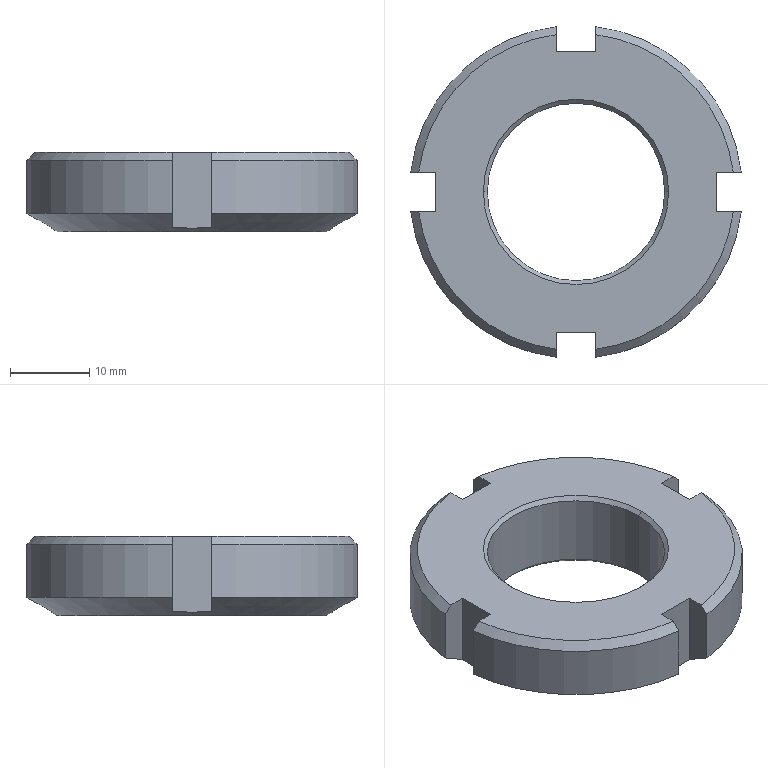Part | SolidWorks | features Chamfer 3, CirPattern 1, Cut 1, Extrusion 1 | 1 solid | 30 faces | box 41.701 x 41.701 x 10 mm | volume 8727 mm3 | plane 14 | cone 10 | cylinder 6 | commonest cylinder face diameters 42 x4 22.376 x2
STEP:
#1=CARTESIAN_POINT('',(-11.188,0.,9.5));
#2=VERTEX_POINT('',#1);
#3=CARTESIAN_POINT('',(11.188,0.,9.5));
#4=VERTEX_POINT('',#3);
#5=CARTESIAN_POINT('',(0.,0.,9.5));
#6=DIRECTION('',(0.,0.,1.));
#7=DIRECTION('',(1.,0.,0.));
#8=AXIS2_PLACEMENT_3D('',#5,#6,#7);
#9=CIRCLE('',#8,11.188);
#10=EDGE_CURVE('',#2,#4,#9,.T.);
#11=ORIENTED_EDGE('',*,*,#10,.F.);
#12=CARTESIAN_POINT('',(-11.688,0.,10.));
#13=VERTEX_POINT('',#12);
#14=CARTESIAN_POINT('',(-11.188,0.,9.5));
#15=DIRECTION('',(-0.7071,0.,0.7071));
#16=VECTOR('',#15,1000.);
#17=LINE('',#14,#16);
#18=EDGE_CURVE('',#2,#13,#17,.T.);
#19=ORIENTED_EDGE('',*,*,#18,.T.);
#20=CARTESIAN_POINT('',(11.688,0.,10.));
#21=VERTEX_POINT('',#20);
#22=CARTESIAN_POINT('',(0.,0.,10.));
#23=DIRECTION('',(0.,0.,-1.));
#24=DIRECTION('',(1.,0.,0.));
#25=AXIS2_PLACEMENT_3D('',#22,#23,#24);
#26=CIRCLE('',#25,11.688);
#27=EDGE_CURVE('',#21,#13,#26,.T.);
#28=ORIENTED_EDGE('',*,*,#27,.F.);
#29=CARTESIAN_POINT('',(11.188,0.,9.5));
#30=DIRECTION('',(0.7071,0.,0.7071));
#31=VECTOR('',#30,1000.);
#32=LINE('',#29,#31);
#33=EDGE_CURVE('',#4,#21,#32,.T.);
#34=ORIENTED_EDGE('',*,*,#33,.F.);
#35=EDGE_LOOP('',(#11,#19,#28,#34));
#36=FACE_OUTER_BOUND('',#35,.T.);
#37=CARTESIAN_POINT('',(0.,0.,9.5));
#38=DIRECTION('',(0.,0.,1.));
#39=DIRECTION('',(1.,0.,0.));
#40=AXIS2_PLACEMENT_3D('',#37,#38,#39);
#41=CONICAL_SURFACE('',#40,11.188,0.7854);
#42=ADVANCED_FACE('',(#36),#41,.F.);
#43=CARTESIAN_POINT('',(11.188,0.,0.5));
#44=VERTEX_POINT('',#43);
#45=CARTESIAN_POINT('',(-11.188,0.,0.5));
#46=VERTEX_POINT('',#45);
#47=CARTESIAN_POINT('',(0.,0.,0.5));
#48=DIRECTION('',(0.,0.,-1.));
#49=DIRECTION('',(1.,0.,0.));
#50=AXIS2_PLACEMENT_3D('',#47,#48,#49);
#51=CIRCLE('',#50,11.188);
#52=EDGE_CURVE('',#44,#46,#51,.T.);
#53=ORIENTED_EDGE('',*,*,#52,.F.);
#54=CARTESIAN_POINT('',(11.688,0.,0.));
#55=VERTEX_POINT('',#54);
#56=CARTESIAN_POINT('',(11.688,0.,0.));
#57=DIRECTION('',(0.7071,0.,-0.7071));
#58=VECTOR('',#57,1000.);
#59=LINE('',#56,#58);
#60=EDGE_CURVE('',#44,#55,#59,.T.);
#61=ORIENTED_EDGE('',*,*,#60,.T.);
#62=CARTESIAN_POINT('',(-11.688,0.,0.));
#63=VERTEX_POINT('',#62);
#64=CARTESIAN_POINT('',(0.,0.,0.));
#65=DIRECTION('',(0.,0.,1.));
#66=DIRECTION('',(1.,0.,0.));
#67=AXIS2_PLACEMENT_3D('',#64,#65,#66);
#68=CIRCLE('',#67,11.688);
#69=EDGE_CURVE('',#63,#55,#68,.T.);
#70=ORIENTED_EDGE('',*,*,#69,.F.);
#71=CARTESIAN_POINT('',(-11.688,0.,0.));
#72=DIRECTION('',(-0.7071,0.,-0.7071));
#73=VECTOR('',#72,1000.);
#74=LINE('',#71,#73);
#75=EDGE_CURVE('',#46,#63,#74,.T.);
#76=ORIENTED_EDGE('',*,*,#75,.F.);
#77=EDGE_LOOP('',(#53,#61,#70,#76));
#78=FACE_OUTER_BOUND('',#77,.T.);
#79=CARTESIAN_POINT('',(0.,0.,0.));
#80=DIRECTION('',(0.,0.,-1.));
#81=DIRECTION('',(-1.,0.,0.));
#82=AXIS2_PLACEMENT_3D('',#79,#80,#81);
#83=CONICAL_SURFACE('',#82,11.688,0.7854);
#84=ADVANCED_FACE('',(#78),#83,.F.);
#85=CARTESIAN_POINT('',(-17.,0.,0.));
#86=VERTEX_POINT('',#85);
#87=CARTESIAN_POINT('',(17.,0.,0.));
#88=VERTEX_POINT('',#87);
#89=CARTESIAN_POINT('',(0.,0.,0.));
#90=DIRECTION('',(0.,0.,-1.));
#91=DIRECTION('',(1.,0.,0.));
#92=AXIS2_PLACEMENT_3D('',#89,#90,#91);
#93=CIRCLE('',#92,17.);
#94=EDGE_CURVE('',#86,#88,#93,.T.);
#95=ORIENTED_EDGE('',*,*,#94,.F.);
#96=CARTESIAN_POINT('',(-17.751,0.,0.4334));
#97=VERTEX_POINT('',#96);
#98=CARTESIAN_POINT('',(-21.,0.,2.309));
#99=DIRECTION('',(-0.866,0.,0.5));
#100=VECTOR('',#99,1000.);
#101=LINE('',#98,#100);
#102=EDGE_CURVE('',#86,#97,#101,.T.);
#103=ORIENTED_EDGE('',*,*,#102,.T.);
#104=CARTESIAN_POINT('',(-17.751,2.5,0.5345));
#105=VERTEX_POINT('',#104);
#106=CARTESIAN_POINT('',(-17.751,2.5,0.5345));
#107=CARTESIAN_POINT('',(-17.751,1.67,0.4677));
#108=CARTESIAN_POINT('',(-17.751,0.8364,0.4334));
#109=CARTESIAN_POINT('',(-17.751,0.,0.4334));
#110=B_SPLINE_CURVE_WITH_KNOTS('',3,(#106,#107,#108,#109),.UNSPECIFIED.,.F.,.F.,(4,4),(0.005311,0.00781),.UNSPECIFIED.);
#111=EDGE_CURVE('',#105,#97,#110,.T.);
#112=ORIENTED_EDGE('',*,*,#111,.F.);
#113=CARTESIAN_POINT('',(-20.851,2.5,2.309));
#114=VERTEX_POINT('',#113);
#115=CARTESIAN_POINT('',(-20.851,2.5,2.309));
#116=CARTESIAN_POINT('',(-19.818,2.5,1.717));
#117=CARTESIAN_POINT('',(-18.784,2.5,1.126));
#118=CARTESIAN_POINT('',(-17.751,2.5,0.5345));
#119=B_SPLINE_CURVE_WITH_KNOTS('',3,(#115,#116,#117,#118),.UNSPECIFIED.,.F.,.F.,(4,4),(0.00673,0.0103),.UNSPECIFIED.);
#120=EDGE_CURVE('',#114,#105,#119,.T.);
#121=ORIENTED_EDGE('',*,*,#120,.F.);
#122=CARTESIAN_POINT('',(-2.5,20.851,2.309));
#123=VERTEX_POINT('',#122);
#124=CARTESIAN_POINT('',(0.,0.,2.309));
#125=DIRECTION('',(0.,0.,1.));
#126=DIRECTION('',(1.,0.,0.));
#127=AXIS2_PLACEMENT_3D('',#124,#125,#126);
#128=CIRCLE('',#127,21.);
#129=EDGE_CURVE('',#123,#114,#128,.T.);
#130=ORIENTED_EDGE('',*,*,#129,.F.);
#131=CARTESIAN_POINT('',(-2.5,17.751,0.5345));
#132=VERTEX_POINT('',#131);
#133=CARTESIAN_POINT('',(-2.5,17.751,0.5345));
#134=CARTESIAN_POINT('',(-2.5,18.784,1.126));
#135=CARTESIAN_POINT('',(-2.5,19.818,1.717));
#136=CARTESIAN_POINT('',(-2.5,20.851,2.309));
#137=B_SPLINE_CURVE_WITH_KNOTS('',3,(#133,#134,#135,#136),.UNSPECIFIED.,.F.,.F.,(4,4),(0.006996,0.01057),.UNSPECIFIED.);
#138=EDGE_CURVE('',#132,#123,#137,.T.);
#139=ORIENTED_EDGE('',*,*,#138,.F.);
#140=CARTESIAN_POINT('',(2.5,17.751,0.5345));
#141=VERTEX_POINT('',#140);
#142=CARTESIAN_POINT('',(2.5,17.751,0.5345));
#143=CARTESIAN_POINT('',(1.672,17.751,0.4679));
#144=CARTESIAN_POINT('',(0.8419,17.751,0.4336));
#145=CARTESIAN_POINT('',(-0.8253,17.751,0.4332));
#146=CARTESIAN_POINT('',(-1.665,17.751,0.4673));
#147=CARTESIAN_POINT('',(-2.5,17.751,0.5345));
#148=B_SPLINE_CURVE_WITH_KNOTS('',3,(#142,#143,#144,#145,#146,#147),.UNSPECIFIED.,.F.,.F.,(4,2,4),(0.005311,0.007801,0.01029),.UNSPECIFIED.);
#149=EDGE_CURVE('',#141,#132,#148,.T.);
#150=ORIENTED_EDGE('',*,*,#149,.F.);
#151=CARTESIAN_POINT('',(2.5,20.851,2.309));
#152=VERTEX_POINT('',#151);
#153=CARTESIAN_POINT('',(2.5,20.851,2.309));
#154=CARTESIAN_POINT('',(2.5,19.818,1.717));
#155=CARTESIAN_POINT('',(2.5,18.784,1.126));
#156=CARTESIAN_POINT('',(2.5,17.751,0.5345));
#157=B_SPLINE_CURVE_WITH_KNOTS('',3,(#153,#154,#155,#156),.UNSPECIFIED.,.F.,.F.,(4,4),(0.004139,0.007711),.UNSPECIFIED.);
#158=EDGE_CURVE('',#152,#141,#157,.T.);
#159=ORIENTED_EDGE('',*,*,#158,.F.);
#160=CARTESIAN_POINT('',(20.851,2.5,2.309));
#161=VERTEX_POINT('',#160);
#162=CARTESIAN_POINT('',(0.,0.,2.309));
#163=DIRECTION('',(0.,0.,1.));
#164=DIRECTION('',(1.,0.,0.));
#165=AXIS2_PLACEMENT_3D('',#162,#163,#164);
#166=CIRCLE('',#165,21.);
#167=EDGE_CURVE('',#161,#152,#166,.T.);
#168=ORIENTED_EDGE('',*,*,#167,.F.);
#169=CARTESIAN_POINT('',(17.751,2.5,0.5345));
#170=VERTEX_POINT('',#169);
#171=CARTESIAN_POINT('',(17.751,2.5,0.5345));
#172=CARTESIAN_POINT('',(18.784,2.5,1.126));
#173=CARTESIAN_POINT('',(19.818,2.5,1.717));
#174=CARTESIAN_POINT('',(20.851,2.5,2.309));
#175=B_SPLINE_CURVE_WITH_KNOTS('',3,(#171,#172,#173,#174),.UNSPECIFIED.,.F.,.F.,(4,4),(0.006996,0.01057),.UNSPECIFIED.);
#176=EDGE_CURVE('',#170,#161,#175,.T.);
#177=ORIENTED_EDGE('',*,*,#176,.F.);
#178=CARTESIAN_POINT('',(17.751,0.,0.4334));
#179=VERTEX_POINT('',#178);
#180=CARTESIAN_POINT('',(17.751,0.,0.4334));
#181=CARTESIAN_POINT('',(17.751,0.8364,0.4334));
#182=CARTESIAN_POINT('',(17.751,1.67,0.4677));
#183=CARTESIAN_POINT('',(17.751,2.5,0.5345));
#184=B_SPLINE_CURVE_WITH_KNOTS('',3,(#180,#181,#182,#183),.UNSPECIFIED.,.F.,.F.,(4,4),(0.01298,0.01548),.UNSPECIFIED.);
#185=EDGE_CURVE('',#179,#170,#184,.T.);
#186=ORIENTED_EDGE('',*,*,#185,.F.);
#187=CARTESIAN_POINT('',(21.,0.,2.309));
#188=DIRECTION('',(0.866,0.,0.5));
#189=VECTOR('',#188,1000.);
#190=LINE('',#187,#189);
#191=EDGE_CURVE('',#88,#179,#190,.T.);
#192=ORIENTED_EDGE('',*,*,#191,.F.);
#193=EDGE_LOOP('',(#95,#103,#112,#121,#130,#139,#150,#159,#168,#177,#186,#192));
#194=FACE_OUTER_BOUND('',#193,.T.);
#195=CARTESIAN_POINT('',(0.,0.,2.309));
#196=DIRECTION('',(0.,0.,1.));
#197=DIRECTION('',(1.,0.,0.));
#198=AXIS2_PLACEMENT_3D('',#195,#196,#197);
#199=CONICAL_SURFACE('',#198,21.,1.047);
#200=ADVANCED_FACE('',(#194),#199,.T.);
#201=ORIENTED_EDGE('',*,*,#10,.T.);
#202=CARTESIAN_POINT('',(11.188,0.,10.));
#203=DIRECTION('',(0.,0.,-1.));
#204=VECTOR('',#203,1000.);
#205=LINE('',#202,#204);
#206=EDGE_CURVE('',#4,#44,#205,.T.);
#207=ORIENTED_EDGE('',*,*,#206,.T.);
#208=ORIENTED_EDGE('',*,*,#52,.T.);
#209=CARTESIAN_POINT('',(-11.188,0.,10.));
#210=DIRECTION('',(0.,0.,-1.));
#211=VECTOR('',#210,1000.);
#212=LINE('',#209,#211);
#213=EDGE_CURVE('',#2,#46,#212,.T.);
#214=ORIENTED_EDGE('',*,*,#213,.F.);
#215=EDGE_LOOP('',(#201,#207,#208,#214));
#216=FACE_OUTER_BOUND('',#215,.T.);
#217=CARTESIAN_POINT('',(0.,0.,10.));
#218=DIRECTION('',(0.,0.,-1.));
#219=DIRECTION('',(-1.,0.,0.));
#220=AXIS2_PLACEMENT_3D('',#217,#218,#219);
#221=CYLINDRICAL_SURFACE('',#220,11.188);
#222=ADVANCED_FACE('',(#216),#221,.F.);
#223=CARTESIAN_POINT('',(2.5,20.851,9.));
#224=VERTEX_POINT('',#223);
#225=CARTESIAN_POINT('',(20.851,2.5,9.));
#226=VERTEX_POINT('',#225);
#227=CARTESIAN_POINT('',(0.,0.,9.));
#228=DIRECTION('',(0.,0.,-1.));
#229=DIRECTION('',(1.,0.,0.));
#230=AXIS2_PLACEMENT_3D('',#227,#228,#229);
#231=CIRCLE('',#230,21.);
#232=EDGE_CURVE('',#224,#226,#231,.T.);
#233=ORIENTED_EDGE('',*,*,#232,.T.);
#234=CARTESIAN_POINT('',(20.851,2.5,0.));
#235=DIRECTION('',(0.,0.,1.));
#236=VECTOR('',#235,1000.);
#237=LINE('',#234,#236);
#238=EDGE_CURVE('',#161,#226,#237,.T.);
#239=ORIENTED_EDGE('',*,*,#238,.F.);
#240=ORIENTED_EDGE('',*,*,#167,.T.);
#241=CARTESIAN_POINT('',(2.5,20.851,0.));
#242=DIRECTION('',(0.,0.,1.));
#243=VECTOR('',#242,1000.);
#244=LINE('',#241,#243);
#245=EDGE_CURVE('',#152,#224,#244,.T.);
#246=ORIENTED_EDGE('',*,*,#245,.T.);
#247=EDGE_LOOP('',(#233,#239,#240,#246));
#248=FACE_OUTER_BOUND('',#247,.T.);
#249=CARTESIAN_POINT('',(0.,0.,10.));
#250=DIRECTION('',(0.,0.,-1.));
#251=DIRECTION('',(-1.,0.,0.));
#252=AXIS2_PLACEMENT_3D('',#249,#250,#251);
#253=CYLINDRICAL_SURFACE('',#252,21.);
#254=ADVANCED_FACE('',(#248),#253,.T.);
#255=CARTESIAN_POINT('',(19.843,2.5,10.));
#256=VERTEX_POINT('',#255);
#257=CARTESIAN_POINT('',(20.851,2.5,9.));
#258=CARTESIAN_POINT('',(20.572,2.5,9.277));
#259=CARTESIAN_POINT('',(20.294,2.5,9.553));
#260=CARTESIAN_POINT('',(20.015,2.5,9.829));
#261=CARTESIAN_POINT('',(19.958,2.5,9.886));
#262=CARTESIAN_POINT('',(19.9,2.5,9.943));
#263=CARTESIAN_POINT('',(19.843,2.5,10.));
#264=B_SPLINE_CURVE_WITH_KNOTS('',3,(#257,#258,#259,#260,#261,#262,#263),.UNSPECIFIED.,.F.,.F.,(4,3,4),(0.005158,0.006335,0.006577),.UNSPECIFIED.);
#265=EDGE_CURVE('',#226,#256,#264,.T.);
#266=ORIENTED_EDGE('',*,*,#265,.F.);
#267=ORIENTED_EDGE('',*,*,#232,.F.);
#268=CARTESIAN_POINT('',(2.5,19.843,10.));
#269=VERTEX_POINT('',#268);
#270=CARTESIAN_POINT('',(2.5,19.843,10.));
#271=CARTESIAN_POINT('',(2.5,19.9,9.943));
#272=CARTESIAN_POINT('',(2.5,19.958,9.886));
#273=CARTESIAN_POINT('',(2.5,20.015,9.829));
#274=CARTESIAN_POINT('',(2.5,20.294,9.553));
#275=CARTESIAN_POINT('',(2.5,20.572,9.277));
#276=CARTESIAN_POINT('',(2.5,20.851,9.));
#277=B_SPLINE_CURVE_WITH_KNOTS('',3,(#270,#271,#272,#273,#274,#275,#276),.UNSPECIFIED.,.F.,.F.,(4,3,4),(0.006093,0.006335,0.007513),.UNSPECIFIED.);
#278=EDGE_CURVE('',#269,#224,#277,.T.);
#279=ORIENTED_EDGE('',*,*,#278,.F.);
#280=CARTESIAN_POINT('',(0.,0.,10.));
#281=DIRECTION('',(0.,0.,1.));
#282=DIRECTION('',(1.,0.,0.));
#283=AXIS2_PLACEMENT_3D('',#280,#281,#282);
#284=CIRCLE('',#283,20.);
#285=EDGE_CURVE('',#256,#269,#284,.T.);
#286=ORIENTED_EDGE('',*,*,#285,.F.);
#287=EDGE_LOOP('',(#266,#267,#279,#286));
#288=FACE_OUTER_BOUND('',#287,.T.);
#289=CARTESIAN_POINT('',(0.,0.,10.));
#290=DIRECTION('',(0.,0.,-1.));
#291=DIRECTION('',(-1.,0.,0.));
#292=AXIS2_PLACEMENT_3D('',#289,#290,#291);
#293=CONICAL_SURFACE('',#292,20.,0.7854);
#294=ADVANCED_FACE('',(#288),#293,.T.);
#295=CARTESIAN_POINT('',(-20.851,2.5,9.));
#296=VERTEX_POINT('',#295);
#297=CARTESIAN_POINT('',(-2.5,20.851,9.));
#298=VERTEX_POINT('',#297);
#299=CARTESIAN_POINT('',(0.,0.,9.));
#300=DIRECTION('',(0.,0.,-1.));
#301=DIRECTION('',(1.,0.,0.));
#302=AXIS2_PLACEMENT_3D('',#299,#300,#301);
#303=CIRCLE('',#302,21.);
#304=EDGE_CURVE('',#296,#298,#303,.T.);
#305=ORIENTED_EDGE('',*,*,#304,.T.);
#306=CARTESIAN_POINT('',(-2.5,20.851,0.));
#307=DIRECTION('',(0.,0.,1.));
#308=VECTOR('',#307,1000.);
#309=LINE('',#306,#308);
#310=EDGE_CURVE('',#123,#298,#309,.T.);
#311=ORIENTED_EDGE('',*,*,#310,.F.);
#312=ORIENTED_EDGE('',*,*,#129,.T.);
#313=CARTESIAN_POINT('',(-20.851,2.5,0.));
#314=DIRECTION('',(0.,0.,1.));
#315=VECTOR('',#314,1000.);
#316=LINE('',#313,#315);
#317=EDGE_CURVE('',#114,#296,#316,.T.);
#318=ORIENTED_EDGE('',*,*,#317,.T.);
#319=EDGE_LOOP('',(#305,#311,#312,#318));
#320=FACE_OUTER_BOUND('',#319,.T.);
#321=CARTESIAN_POINT('',(0.,0.,10.));
#322=DIRECTION('',(0.,0.,-1.));
#323=DIRECTION('',(-1.,0.,0.));
#324=AXIS2_PLACEMENT_3D('',#321,#322,#323);
#325=CYLINDRICAL_SURFACE('',#324,21.);
#326=ADVANCED_FACE('',(#320),#325,.T.);
#327=CARTESIAN_POINT('',(-2.5,19.843,10.));
#328=VERTEX_POINT('',#327);
#329=CARTESIAN_POINT('',(-2.5,20.851,9.));
#330=CARTESIAN_POINT('',(-2.5,20.572,9.277));
#331=CARTESIAN_POINT('',(-2.5,20.294,9.553));
#332=CARTESIAN_POINT('',(-2.5,20.015,9.829));
#333=CARTESIAN_POINT('',(-2.5,19.958,9.886));
#334=CARTESIAN_POINT('',(-2.5,19.9,9.943));
#335=CARTESIAN_POINT('',(-2.5,19.843,10.));
#336=B_SPLINE_CURVE_WITH_KNOTS('',3,(#329,#330,#331,#332,#333,#334,#335),.UNSPECIFIED.,.F.,.F.,(4,3,4),(0.005158,0.006335,0.006577),.UNSPECIFIED.);
#337=EDGE_CURVE('',#298,#328,#336,.T.);
#338=ORIENTED_EDGE('',*,*,#337,.F.);
#339=ORIENTED_EDGE('',*,*,#304,.F.);
#340=CARTESIAN_POINT('',(-19.843,2.5,10.));
#341=VERTEX_POINT('',#340);
#342=CARTESIAN_POINT('',(-19.843,2.5,10.));
#343=CARTESIAN_POINT('',(-20.031,2.5,9.814));
#344=CARTESIAN_POINT('',(-20.218,2.5,9.628));
#345=CARTESIAN_POINT('',(-20.406,2.5,9.442));
#346=CARTESIAN_POINT('',(-20.554,2.5,9.295));
#347=CARTESIAN_POINT('',(-20.702,2.5,9.147));
#348=CARTESIAN_POINT('',(-20.851,2.5,9.));
#349=B_SPLINE_CURVE_WITH_KNOTS('',3,(#342,#343,#344,#345,#346,#347,#348),.UNSPECIFIED.,.F.,.F.,(4,3,4),(0.005543,0.006335,0.006963),.UNSPECIFIED.);
#350=EDGE_CURVE('',#341,#296,#349,.T.);
#351=ORIENTED_EDGE('',*,*,#350,.F.);
#352=CARTESIAN_POINT('',(0.,0.,10.));
#353=DIRECTION('',(0.,0.,1.));
#354=DIRECTION('',(1.,0.,0.));
#355=AXIS2_PLACEMENT_3D('',#352,#353,#354);
#356=CIRCLE('',#355,20.);
#357=EDGE_CURVE('',#328,#341,#356,.T.);
#358=ORIENTED_EDGE('',*,*,#357,.F.);
#359=EDGE_LOOP('',(#338,#339,#351,#358));
#360=FACE_OUTER_BOUND('',#359,.T.);
#361=CARTESIAN_POINT('',(0.,0.,10.));
#362=DIRECTION('',(0.,0.,-1.));
#363=DIRECTION('',(-1.,0.,0.));
#364=AXIS2_PLACEMENT_3D('',#361,#362,#363);
#365=CONICAL_SURFACE('',#364,20.,0.7854);
#366=ADVANCED_FACE('',(#360),#365,.T.);
#367=CARTESIAN_POINT('',(-2.5,-20.851,9.));
#368=VERTEX_POINT('',#367);
#369=CARTESIAN_POINT('',(-20.851,-2.5,9.));
#370=VERTEX_POINT('',#369);
#371=CARTESIAN_POINT('',(0.,0.,9.));
#372=DIRECTION('',(0.,0.,-1.));
#373=DIRECTION('',(1.,0.,0.));
#374=AXIS2_PLACEMENT_3D('',#371,#372,#373);
#375=CIRCLE('',#374,21.);
#376=EDGE_CURVE('',#368,#370,#375,.T.);
#377=ORIENTED_EDGE('',*,*,#376,.T.);
#378=CARTESIAN_POINT('',(-20.851,-2.5,2.309));
#379=VERTEX_POINT('',#378);
#380=CARTESIAN_POINT('',(-20.851,-2.5,0.));
#381=DIRECTION('',(0.,0.,1.));
#382=VECTOR('',#381,1000.);
#383=LINE('',#380,#382);
#384=EDGE_CURVE('',#379,#370,#383,.T.);
#385=ORIENTED_EDGE('',*,*,#384,.F.);
#386=CARTESIAN_POINT('',(-2.5,-20.851,2.309));
#387=VERTEX_POINT('',#386);
#388=CARTESIAN_POINT('',(0.,0.,2.309));
#389=DIRECTION('',(0.,0.,1.));
#390=DIRECTION('',(1.,0.,0.));
#391=AXIS2_PLACEMENT_3D('',#388,#389,#390);
#392=CIRCLE('',#391,21.);
#393=EDGE_CURVE('',#379,#387,#392,.T.);
#394=ORIENTED_EDGE('',*,*,#393,.T.);
#395=CARTESIAN_POINT('',(-2.5,-20.851,0.));
#396=DIRECTION('',(0.,0.,1.));
#397=VECTOR('',#396,1000.);
#398=LINE('',#395,#397);
#399=EDGE_CURVE('',#387,#368,#398,.T.);
#400=ORIENTED_EDGE('',*,*,#399,.T.);
#401=EDGE_LOOP('',(#377,#385,#394,#400));
#402=FACE_OUTER_BOUND('',#401,.T.);
#403=CARTESIAN_POINT('',(0.,0.,10.));
#404=DIRECTION('',(0.,0.,-1.));
#405=DIRECTION('',(-1.,0.,0.));
#406=AXIS2_PLACEMENT_3D('',#403,#404,#405);
#407=CYLINDRICAL_SURFACE('',#406,21.);
#408=ADVANCED_FACE('',(#402),#407,.T.);
#409=CARTESIAN_POINT('',(-19.843,-2.5,10.));
#410=VERTEX_POINT('',#409);
#411=CARTESIAN_POINT('',(-20.851,-2.5,9.));
#412=CARTESIAN_POINT('',(-20.702,-2.5,9.147));
#413=CARTESIAN_POINT('',(-20.554,-2.5,9.295));
#414=CARTESIAN_POINT('',(-20.406,-2.5,9.442));
#415=CARTESIAN_POINT('',(-20.218,-2.5,9.628));
#416=CARTESIAN_POINT('',(-20.031,-2.5,9.814));
#417=CARTESIAN_POINT('',(-19.843,-2.5,10.));
#418=B_SPLINE_CURVE_WITH_KNOTS('',3,(#411,#412,#413,#414,#415,#416,#417),.UNSPECIFIED.,.F.,.F.,(4,3,4),(0.005708,0.006335,0.007128),.UNSPECIFIED.);
#419=EDGE_CURVE('',#370,#410,#418,.T.);
#420=ORIENTED_EDGE('',*,*,#419,.F.);
#421=ORIENTED_EDGE('',*,*,#376,.F.);
#422=CARTESIAN_POINT('',(-2.5,-19.843,10.));
#423=VERTEX_POINT('',#422);
#424=CARTESIAN_POINT('',(-2.5,-19.843,10.));
#425=CARTESIAN_POINT('',(-2.5,-20.031,9.814));
#426=CARTESIAN_POINT('',(-2.5,-20.218,9.628));
#427=CARTESIAN_POINT('',(-2.5,-20.406,9.442));
#428=CARTESIAN_POINT('',(-2.5,-20.554,9.295));
#429=CARTESIAN_POINT('',(-2.5,-20.702,9.147));
#430=CARTESIAN_POINT('',(-2.5,-20.851,9.));
#431=B_SPLINE_CURVE_WITH_KNOTS('',3,(#424,#425,#426,#427,#428,#429,#430),.UNSPECIFIED.,.F.,.F.,(4,3,4),(0.005543,0.006335,0.006963),.UNSPECIFIED.);
#432=EDGE_CURVE('',#423,#368,#431,.T.);
#433=ORIENTED_EDGE('',*,*,#432,.F.);
#434=CARTESIAN_POINT('',(0.,0.,10.));
#435=DIRECTION('',(0.,0.,1.));
#436=DIRECTION('',(1.,0.,0.));
#437=AXIS2_PLACEMENT_3D('',#434,#435,#436);
#438=CIRCLE('',#437,20.);
#439=EDGE_CURVE('',#410,#423,#438,.T.);
#440=ORIENTED_EDGE('',*,*,#439,.F.);
#441=EDGE_LOOP('',(#420,#421,#433,#440));
#442=FACE_OUTER_BOUND('',#441,.T.);
#443=CARTESIAN_POINT('',(0.,0.,10.));
#444=DIRECTION('',(0.,0.,-1.));
#445=DIRECTION('',(-1.,0.,0.));
#446=AXIS2_PLACEMENT_3D('',#443,#444,#445);
#447=CONICAL_SURFACE('',#446,20.,0.7854);
#448=ADVANCED_FACE('',(#442),#447,.T.);
#449=ORIENTED_EDGE('',*,*,#27,.T.);
#450=CARTESIAN_POINT('',(0.,0.,10.));
#451=DIRECTION('',(0.,0.,-1.));
#452=DIRECTION('',(1.,0.,0.));
#453=AXIS2_PLACEMENT_3D('',#450,#451,#452);
#454=CIRCLE('',#453,11.688);
#455=EDGE_CURVE('',#13,#21,#454,.T.);
#456=ORIENTED_EDGE('',*,*,#455,.T.);
#457=EDGE_LOOP('',(#449,#456));
#458=FACE_BOUND('',#457,.T.);
#459=CARTESIAN_POINT('',(17.751,2.5,10.));
#460=VERTEX_POINT('',#459);
#461=CARTESIAN_POINT('',(17.751,2.5,10.));
#462=DIRECTION('',(-1.,0.,0.));
#463=VECTOR('',#462,1000.);
#464=LINE('',#461,#463);
#465=EDGE_CURVE('',#256,#460,#464,.T.);
#466=ORIENTED_EDGE('',*,*,#465,.F.);
#467=ORIENTED_EDGE('',*,*,#285,.T.);
#468=CARTESIAN_POINT('',(2.5,17.751,10.));
#469=VERTEX_POINT('',#468);
#470=CARTESIAN_POINT('',(2.5,17.751,10.));
#471=DIRECTION('',(0.,1.,0.));
#472=VECTOR('',#471,1000.);
#473=LINE('',#470,#472);
#474=EDGE_CURVE('',#469,#269,#473,.T.);
#475=ORIENTED_EDGE('',*,*,#474,.F.);
#476=CARTESIAN_POINT('',(-2.5,17.751,10.));
#477=VERTEX_POINT('',#476);
#478=CARTESIAN_POINT('',(2.5,17.751,10.));
#479=DIRECTION('',(1.,0.,0.));
#480=VECTOR('',#479,1000.);
#481=LINE('',#478,#480);
#482=EDGE_CURVE('',#477,#469,#481,.T.);
#483=ORIENTED_EDGE('',*,*,#482,.F.);
#484=CARTESIAN_POINT('',(-2.5,17.751,10.));
#485=DIRECTION('',(0.,-1.,0.));
#486=VECTOR('',#485,1000.);
#487=LINE('',#484,#486);
#488=EDGE_CURVE('',#328,#477,#487,.T.);
#489=ORIENTED_EDGE('',*,*,#488,.F.);
#490=ORIENTED_EDGE('',*,*,#357,.T.);
#491=CARTESIAN_POINT('',(-17.751,2.5,10.));
#492=VERTEX_POINT('',#491);
#493=CARTESIAN_POINT('',(-17.751,2.5,10.));
#494=DIRECTION('',(-1.,0.,0.));
#495=VECTOR('',#494,1000.);
#496=LINE('',#493,#495);
#497=EDGE_CURVE('',#492,#341,#496,.T.);
#498=ORIENTED_EDGE('',*,*,#497,.F.);
#499=CARTESIAN_POINT('',(-17.751,-2.5,10.));
#500=VERTEX_POINT('',#499);
#501=CARTESIAN_POINT('',(-17.751,2.5,10.));
#502=DIRECTION('',(0.,1.,0.));
#503=VECTOR('',#502,1000.);
#504=LINE('',#501,#503);
#505=EDGE_CURVE('',#500,#492,#504,.T.);
#506=ORIENTED_EDGE('',*,*,#505,.F.);
#507=CARTESIAN_POINT('',(-17.751,-2.5,10.));
#508=DIRECTION('',(1.,0.,0.));
#509=VECTOR('',#508,1000.);
#510=LINE('',#507,#509);
#511=EDGE_CURVE('',#410,#500,#510,.T.);
#512=ORIENTED_EDGE('',*,*,#511,.F.);
#513=ORIENTED_EDGE('',*,*,#439,.T.);
#514=CARTESIAN_POINT('',(-2.5,-17.751,10.));
#515=VERTEX_POINT('',#514);
#516=CARTESIAN_POINT('',(-2.5,-17.751,10.));
#517=DIRECTION('',(0.,-1.,0.));
#518=VECTOR('',#517,1000.);
#519=LINE('',#516,#518);
#520=EDGE_CURVE('',#515,#423,#519,.T.);
#521=ORIENTED_EDGE('',*,*,#520,.F.);
#522=CARTESIAN_POINT('',(2.5,-17.751,10.));
#523=VERTEX_POINT('',#522);
#524=CARTESIAN_POINT('',(-2.5,-17.751,10.));
#525=DIRECTION('',(-1.,0.,0.));
#526=VECTOR('',#525,1000.);
#527=LINE('',#524,#526);
#528=EDGE_CURVE('',#523,#515,#527,.T.);
#529=ORIENTED_EDGE('',*,*,#528,.F.);
#530=CARTESIAN_POINT('',(2.5,-19.843,10.));
#531=VERTEX_POINT('',#530);
#532=CARTESIAN_POINT('',(2.5,-17.751,10.));
#533=DIRECTION('',(0.,1.,0.));
#534=VECTOR('',#533,1000.);
#535=LINE('',#532,#534);
#536=EDGE_CURVE('',#531,#523,#535,.T.);
#537=ORIENTED_EDGE('',*,*,#536,.F.);
#538=CARTESIAN_POINT('',(19.843,-2.5,10.));
#539=VERTEX_POINT('',#538);
#540=CARTESIAN_POINT('',(0.,0.,10.));
#541=DIRECTION('',(0.,0.,1.));
#542=DIRECTION('',(1.,0.,0.));
#543=AXIS2_PLACEMENT_3D('',#540,#541,#542);
#544=CIRCLE('',#543,20.);
#545=EDGE_CURVE('',#531,#539,#544,.T.);
#546=ORIENTED_EDGE('',*,*,#545,.T.);
#547=CARTESIAN_POINT('',(17.751,-2.5,10.));
#548=VERTEX_POINT('',#547);
#549=CARTESIAN_POINT('',(17.751,-2.5,10.));
#550=DIRECTION('',(1.,0.,0.));
#551=VECTOR('',#550,1000.);
#552=LINE('',#549,#551);
#553=EDGE_CURVE('',#548,#539,#552,.T.);
#554=ORIENTED_EDGE('',*,*,#553,.F.);
#555=CARTESIAN_POINT('',(17.751,-2.5,10.));
#556=DIRECTION('',(0.,-1.,0.));
#557=VECTOR('',#556,1000.);
#558=LINE('',#555,#557);
#559=EDGE_CURVE('',#460,#548,#558,.T.);
#560=ORIENTED_EDGE('',*,*,#559,.F.);
#561=EDGE_LOOP('',(#466,#467,#475,#483,#489,#490,#498,#506,#512,#513,#521,#529,#537,#546,#554,#560));
#562=FACE_OUTER_BOUND('',#561,.T.);
#563=CARTESIAN_POINT('',(0.,0.,10.));
#564=DIRECTION('',(0.,0.,1.));
#565=DIRECTION('',(1.,0.,0.));
#566=AXIS2_PLACEMENT_3D('',#563,#564,#565);
#567=PLANE('',#566);
#568=ADVANCED_FACE('',(#458,#562),#567,.T.);
#569=ORIENTED_EDGE('',*,*,#69,.T.);
#570=CARTESIAN_POINT('',(0.,0.,0.));
#571=DIRECTION('',(0.,0.,1.));
#572=DIRECTION('',(1.,0.,0.));
#573=AXIS2_PLACEMENT_3D('',#570,#571,#572);
#574=CIRCLE('',#573,11.688);
#575=EDGE_CURVE('',#55,#63,#574,.T.);
#576=ORIENTED_EDGE('',*,*,#575,.T.);
#577=EDGE_LOOP('',(#569,#576));
#578=FACE_BOUND('',#577,.T.);
#579=CARTESIAN_POINT('',(0.,0.,0.));
#580=DIRECTION('',(0.,0.,-1.));
#581=DIRECTION('',(1.,0.,0.));
#582=AXIS2_PLACEMENT_3D('',#579,#580,#581);
#583=CIRCLE('',#582,17.);
#584=EDGE_CURVE('',#88,#86,#583,.T.);
#585=ORIENTED_EDGE('',*,*,#584,.T.);
#586=ORIENTED_EDGE('',*,*,#94,.T.);
#587=EDGE_LOOP('',(#585,#586));
#588=FACE_OUTER_BOUND('',#587,.T.);
#589=CARTESIAN_POINT('',(0.,0.,0.));
#590=DIRECTION('',(0.,0.,1.));
#591=DIRECTION('',(1.,0.,0.));
#592=AXIS2_PLACEMENT_3D('',#589,#590,#591);
#593=PLANE('',#592);
#594=ADVANCED_FACE('',(#578,#588),#593,.F.);
#595=CARTESIAN_POINT('',(2.5,-20.851,2.309));
#596=VERTEX_POINT('',#595);
#597=CARTESIAN_POINT('',(20.851,-2.5,2.309));
#598=VERTEX_POINT('',#597);
#599=CARTESIAN_POINT('',(0.,0.,2.309));
#600=DIRECTION('',(0.,0.,1.));
#601=DIRECTION('',(1.,0.,0.));
#602=AXIS2_PLACEMENT_3D('',#599,#600,#601);
#603=CIRCLE('',#602,21.);
#604=EDGE_CURVE('',#596,#598,#603,.T.);
#605=ORIENTED_EDGE('',*,*,#604,.T.);
#606=CARTESIAN_POINT('',(20.851,-2.5,9.));
#607=VERTEX_POINT('',#606);
#608=CARTESIAN_POINT('',(20.851,-2.5,0.));
#609=DIRECTION('',(0.,0.,1.));
#610=VECTOR('',#609,1000.);
#611=LINE('',#608,#610);
#612=EDGE_CURVE('',#598,#607,#611,.T.);
#613=ORIENTED_EDGE('',*,*,#612,.T.);
#614=CARTESIAN_POINT('',(2.5,-20.851,9.));
#615=VERTEX_POINT('',#614);
#616=CARTESIAN_POINT('',(0.,0.,9.));
#617=DIRECTION('',(0.,0.,-1.));
#618=DIRECTION('',(1.,0.,0.));
#619=AXIS2_PLACEMENT_3D('',#616,#617,#618);
#620=CIRCLE('',#619,21.);
#621=EDGE_CURVE('',#607,#615,#620,.T.);
#622=ORIENTED_EDGE('',*,*,#621,.T.);
#623=CARTESIAN_POINT('',(2.5,-20.851,0.));
#624=DIRECTION('',(0.,0.,1.));
#625=VECTOR('',#624,1000.);
#626=LINE('',#623,#625);
#627=EDGE_CURVE('',#596,#615,#626,.T.);
#628=ORIENTED_EDGE('',*,*,#627,.F.);
#629=EDGE_LOOP('',(#605,#613,#622,#628));
#630=FACE_OUTER_BOUND('',#629,.T.);
#631=CARTESIAN_POINT('',(0.,0.,10.));
#632=DIRECTION('',(0.,0.,-1.));
#633=DIRECTION('',(-1.,0.,0.));
#634=AXIS2_PLACEMENT_3D('',#631,#632,#633);
#635=CYLINDRICAL_SURFACE('',#634,21.);
#636=ADVANCED_FACE('',(#630),#635,.T.);
#637=ORIENTED_EDGE('',*,*,#206,.F.);
#638=CARTESIAN_POINT('',(0.,0.,9.5));
#639=DIRECTION('',(0.,0.,1.));
#640=DIRECTION('',(1.,0.,0.));
#641=AXIS2_PLACEMENT_3D('',#638,#639,#640);
#642=CIRCLE('',#641,11.188);
#643=EDGE_CURVE('',#4,#2,#642,.T.);
#644=ORIENTED_EDGE('',*,*,#643,.T.);
#645=ORIENTED_EDGE('',*,*,#213,.T.);
#646=CARTESIAN_POINT('',(0.,0.,0.5));
#647=DIRECTION('',(0.,0.,-1.));
#648=DIRECTION('',(1.,0.,0.));
#649=AXIS2_PLACEMENT_3D('',#646,#647,#648);
#650=CIRCLE('',#649,11.188);
#651=EDGE_CURVE('',#46,#44,#650,.T.);
#652=ORIENTED_EDGE('',*,*,#651,.T.);
#653=EDGE_LOOP('',(#637,#644,#645,#652));
#654=FACE_OUTER_BOUND('',#653,.T.);
#655=CARTESIAN_POINT('',(0.,0.,10.));
#656=DIRECTION('',(0.,0.,-1.));
#657=DIRECTION('',(-1.,0.,0.));
#658=AXIS2_PLACEMENT_3D('',#655,#656,#657);
#659=CYLINDRICAL_SURFACE('',#658,11.188);
#660=ADVANCED_FACE('',(#654),#659,.F.);
#661=CARTESIAN_POINT('',(19.843,-2.5,10.));
#662=CARTESIAN_POINT('',(19.9,-2.5,9.943));
#663=CARTESIAN_POINT('',(19.958,-2.5,9.886));
#664=CARTESIAN_POINT('',(20.015,-2.5,9.829));
#665=CARTESIAN_POINT('',(20.294,-2.5,9.553));
#666=CARTESIAN_POINT('',(20.572,-2.5,9.277));
#667=CARTESIAN_POINT('',(20.851,-2.5,9.));
#668=B_SPLINE_CURVE_WITH_KNOTS('',3,(#661,#662,#663,#664,#665,#666,#667),.UNSPECIFIED.,.F.,.F.,(4,3,4),(0.006093,0.006335,0.007513),.UNSPECIFIED.);
#669=EDGE_CURVE('',#539,#607,#668,.T.);
#670=ORIENTED_EDGE('',*,*,#669,.F.);
#671=ORIENTED_EDGE('',*,*,#545,.F.);
#672=CARTESIAN_POINT('',(2.5,-20.851,9.));
#673=CARTESIAN_POINT('',(2.5,-20.702,9.147));
#674=CARTESIAN_POINT('',(2.5,-20.554,9.295));
#675=CARTESIAN_POINT('',(2.5,-20.406,9.442));
#676=CARTESIAN_POINT('',(2.5,-20.218,9.628));
#677=CARTESIAN_POINT('',(2.5,-20.031,9.814));
#678=CARTESIAN_POINT('',(2.5,-19.843,10.));
#679=B_SPLINE_CURVE_WITH_KNOTS('',3,(#672,#673,#674,#675,#676,#677,#678),.UNSPECIFIED.,.F.,.F.,(4,3,4),(0.005708,0.006335,0.007128),.UNSPECIFIED.);
#680=EDGE_CURVE('',#615,#531,#679,.T.);
#681=ORIENTED_EDGE('',*,*,#680,.F.);
#682=ORIENTED_EDGE('',*,*,#621,.F.);
#683=EDGE_LOOP('',(#670,#671,#681,#682));
#684=FACE_OUTER_BOUND('',#683,.T.);
#685=CARTESIAN_POINT('',(0.,0.,10.));
#686=DIRECTION('',(0.,0.,-1.));
#687=DIRECTION('',(-1.,0.,0.));
#688=AXIS2_PLACEMENT_3D('',#685,#686,#687);
#689=CONICAL_SURFACE('',#688,20.,0.7854);
#690=ADVANCED_FACE('',(#684),#689,.T.);
#691=ORIENTED_EDGE('',*,*,#102,.F.);
#692=ORIENTED_EDGE('',*,*,#584,.F.);
#693=ORIENTED_EDGE('',*,*,#191,.T.);
#694=CARTESIAN_POINT('',(17.751,-2.5,0.5345));
#695=VERTEX_POINT('',#694);
#696=CARTESIAN_POINT('',(17.751,-2.5,0.5345));
#697=CARTESIAN_POINT('',(17.751,-1.668,0.4675));
#698=CARTESIAN_POINT('',(17.751,-0.8309,0.4334));
#699=CARTESIAN_POINT('',(17.751,0.,0.4334));
#700=B_SPLINE_CURVE_WITH_KNOTS('',3,(#696,#697,#698,#699),.UNSPECIFIED.,.F.,.F.,(4,4),(0.0105,0.01298),.UNSPECIFIED.);
#701=EDGE_CURVE('',#695,#179,#700,.T.);
#702=ORIENTED_EDGE('',*,*,#701,.F.);
#703=CARTESIAN_POINT('',(20.851,-2.5,2.309));
#704=CARTESIAN_POINT('',(19.818,-2.5,1.717));
#705=CARTESIAN_POINT('',(18.784,-2.5,1.126));
#706=CARTESIAN_POINT('',(17.751,-2.5,0.5345));
#707=B_SPLINE_CURVE_WITH_KNOTS('',3,(#703,#704,#705,#706),.UNSPECIFIED.,.F.,.F.,(4,4),(0.004139,0.007711),.UNSPECIFIED.);
#708=EDGE_CURVE('',#598,#695,#707,.T.);
#709=ORIENTED_EDGE('',*,*,#708,.F.);
#710=ORIENTED_EDGE('',*,*,#604,.F.);
#711=CARTESIAN_POINT('',(2.5,-17.751,0.5345));
#712=VERTEX_POINT('',#711);
#713=CARTESIAN_POINT('',(2.5,-17.751,0.5345));
#714=CARTESIAN_POINT('',(2.5,-18.784,1.126));
#715=CARTESIAN_POINT('',(2.5,-19.818,1.717));
#716=CARTESIAN_POINT('',(2.5,-20.851,2.309));
#717=B_SPLINE_CURVE_WITH_KNOTS('',3,(#713,#714,#715,#716),.UNSPECIFIED.,.F.,.F.,(4,4),(0.004405,0.007977),.UNSPECIFIED.);
#718=EDGE_CURVE('',#712,#596,#717,.T.);
#719=ORIENTED_EDGE('',*,*,#718,.F.);
#720=CARTESIAN_POINT('',(-2.5,-17.751,0.5345));
#721=VERTEX_POINT('',#720);
#722=CARTESIAN_POINT('',(-2.5,-17.751,0.5345));
#723=CARTESIAN_POINT('',(-1.665,-17.751,0.4673));
#724=CARTESIAN_POINT('',(-0.8253,-17.751,0.4332));
#725=CARTESIAN_POINT('',(0.8419,-17.751,0.4336));
#726=CARTESIAN_POINT('',(1.672,-17.751,0.4679));
#727=CARTESIAN_POINT('',(2.5,-17.751,0.5345));
#728=B_SPLINE_CURVE_WITH_KNOTS('',3,(#722,#723,#724,#725,#726,#727),.UNSPECIFIED.,.F.,.F.,(4,2,4),(0.0105,0.01299,0.01548),.UNSPECIFIED.);
#729=EDGE_CURVE('',#721,#712,#728,.T.);
#730=ORIENTED_EDGE('',*,*,#729,.F.);
#731=CARTESIAN_POINT('',(-2.5,-20.851,2.309));
#732=CARTESIAN_POINT('',(-2.5,-19.818,1.717));
#733=CARTESIAN_POINT('',(-2.5,-18.784,1.126));
#734=CARTESIAN_POINT('',(-2.5,-17.751,0.5345));
#735=B_SPLINE_CURVE_WITH_KNOTS('',3,(#731,#732,#733,#734),.UNSPECIFIED.,.F.,.F.,(4,4),(0.00673,0.0103),.UNSPECIFIED.);
#736=EDGE_CURVE('',#387,#721,#735,.T.);
#737=ORIENTED_EDGE('',*,*,#736,.F.);
#738=ORIENTED_EDGE('',*,*,#393,.F.);
#739=CARTESIAN_POINT('',(-17.751,-2.5,0.5345));
#740=VERTEX_POINT('',#739);
#741=CARTESIAN_POINT('',(-17.751,-2.5,0.5345));
#742=CARTESIAN_POINT('',(-18.784,-2.5,1.126));
#743=CARTESIAN_POINT('',(-19.818,-2.5,1.717));
#744=CARTESIAN_POINT('',(-20.851,-2.5,2.309));
#745=B_SPLINE_CURVE_WITH_KNOTS('',3,(#741,#742,#743,#744),.UNSPECIFIED.,.F.,.F.,(4,4),(0.004405,0.007977),.UNSPECIFIED.);
#746=EDGE_CURVE('',#740,#379,#745,.T.);
#747=ORIENTED_EDGE('',*,*,#746,.F.);
#748=CARTESIAN_POINT('',(-17.751,0.,0.4334));
#749=CARTESIAN_POINT('',(-17.751,-0.8309,0.4334));
#750=CARTESIAN_POINT('',(-17.751,-1.668,0.4675));
#751=CARTESIAN_POINT('',(-17.751,-2.5,0.5345));
#752=B_SPLINE_CURVE_WITH_KNOTS('',3,(#748,#749,#750,#751),.UNSPECIFIED.,.F.,.F.,(4,4),(0.00781,0.01029),.UNSPECIFIED.);
#753=EDGE_CURVE('',#97,#740,#752,.T.);
#754=ORIENTED_EDGE('',*,*,#753,.F.);
#755=EDGE_LOOP('',(#691,#692,#693,#702,#709,#710,#719,#730,#737,#738,#747,#754));
#756=FACE_OUTER_BOUND('',#755,.T.);
#757=CARTESIAN_POINT('',(0.,0.,2.309));
#758=DIRECTION('',(0.,0.,1.));
#759=DIRECTION('',(1.,0.,0.));
#760=AXIS2_PLACEMENT_3D('',#757,#758,#759);
#761=CONICAL_SURFACE('',#760,21.,1.047);
#762=ADVANCED_FACE('',(#756),#761,.T.);
#763=ORIENTED_EDGE('',*,*,#729,.T.);
#764=CARTESIAN_POINT('',(2.5,-17.751,0.));
#765=DIRECTION('',(0.,0.,1.));
#766=VECTOR('',#765,1000.);
#767=LINE('',#764,#766);
#768=EDGE_CURVE('',#712,#523,#767,.T.);
#769=ORIENTED_EDGE('',*,*,#768,.T.);
#770=ORIENTED_EDGE('',*,*,#528,.T.);
#771=CARTESIAN_POINT('',(-2.5,-17.751,0.));
#772=DIRECTION('',(0.,0.,1.));
#773=VECTOR('',#772,1000.);
#774=LINE('',#771,#773);
#775=EDGE_CURVE('',#721,#515,#774,.T.);
#776=ORIENTED_EDGE('',*,*,#775,.F.);
#777=EDGE_LOOP('',(#763,#769,#770,#776));
#778=FACE_OUTER_BOUND('',#777,.T.);
#779=CARTESIAN_POINT('',(-2.5,-17.751,0.));
#780=DIRECTION('',(0.,1.,0.));
#781=DIRECTION('',(0.,0.,1.));
#782=AXIS2_PLACEMENT_3D('',#779,#780,#781);
#783=PLANE('',#782);
#784=ADVANCED_FACE('',(#778),#783,.F.);
#785=ORIENTED_EDGE('',*,*,#680,.T.);
#786=ORIENTED_EDGE('',*,*,#536,.T.);
#787=ORIENTED_EDGE('',*,*,#768,.F.);
#788=ORIENTED_EDGE('',*,*,#718,.T.);
#789=ORIENTED_EDGE('',*,*,#627,.T.);
#790=EDGE_LOOP('',(#785,#786,#787,#788,#789));
#791=FACE_OUTER_BOUND('',#790,.T.);
#792=CARTESIAN_POINT('',(2.5,-17.751,0.));
#793=DIRECTION('',(1.,0.,0.));
#794=DIRECTION('',(0.,1.,0.));
#795=AXIS2_PLACEMENT_3D('',#792,#793,#794);
#796=PLANE('',#795);
#797=ADVANCED_FACE('',(#791),#796,.F.);
#798=ORIENTED_EDGE('',*,*,#432,.T.);
#799=ORIENTED_EDGE('',*,*,#399,.F.);
#800=ORIENTED_EDGE('',*,*,#736,.T.);
#801=ORIENTED_EDGE('',*,*,#775,.T.);
#802=ORIENTED_EDGE('',*,*,#520,.T.);
#803=EDGE_LOOP('',(#798,#799,#800,#801,#802));
#804=FACE_OUTER_BOUND('',#803,.T.);
#805=CARTESIAN_POINT('',(-2.5,-17.751,0.));
#806=DIRECTION('',(-1.,0.,0.));
#807=DIRECTION('',(0.,-1.,0.));
#808=AXIS2_PLACEMENT_3D('',#805,#806,#807);
#809=PLANE('',#808);
#810=ADVANCED_FACE('',(#804),#809,.F.);
#811=ORIENTED_EDGE('',*,*,#111,.T.);
#812=ORIENTED_EDGE('',*,*,#753,.T.);
#813=CARTESIAN_POINT('',(-17.751,-2.5,0.));
#814=DIRECTION('',(0.,0.,1.));
#815=VECTOR('',#814,1000.);
#816=LINE('',#813,#815);
#817=EDGE_CURVE('',#740,#500,#816,.T.);
#818=ORIENTED_EDGE('',*,*,#817,.T.);
#819=ORIENTED_EDGE('',*,*,#505,.T.);
#820=CARTESIAN_POINT('',(-17.751,2.5,0.));
#821=DIRECTION('',(0.,0.,1.));
#822=VECTOR('',#821,1000.);
#823=LINE('',#820,#822);
#824=EDGE_CURVE('',#105,#492,#823,.T.);
#825=ORIENTED_EDGE('',*,*,#824,.F.);
#826=EDGE_LOOP('',(#811,#812,#818,#819,#825));
#827=FACE_OUTER_BOUND('',#826,.T.);
#828=CARTESIAN_POINT('',(-17.751,2.5,0.));
#829=DIRECTION('',(1.,0.,0.));
#830=DIRECTION('',(0.,1.,0.));
#831=AXIS2_PLACEMENT_3D('',#828,#829,#830);
#832=PLANE('',#831);
#833=ADVANCED_FACE('',(#827),#832,.F.);
#834=ORIENTED_EDGE('',*,*,#419,.T.);
#835=ORIENTED_EDGE('',*,*,#511,.T.);
#836=ORIENTED_EDGE('',*,*,#817,.F.);
#837=ORIENTED_EDGE('',*,*,#746,.T.);
#838=ORIENTED_EDGE('',*,*,#384,.T.);
#839=EDGE_LOOP('',(#834,#835,#836,#837,#838));
#840=FACE_OUTER_BOUND('',#839,.T.);
#841=CARTESIAN_POINT('',(-17.751,-2.5,0.));
#842=DIRECTION('',(0.,-1.,0.));
#843=DIRECTION('',(1.,0.,0.));
#844=AXIS2_PLACEMENT_3D('',#841,#842,#843);
#845=PLANE('',#844);
#846=ADVANCED_FACE('',(#840),#845,.F.);
#847=ORIENTED_EDGE('',*,*,#350,.T.);
#848=ORIENTED_EDGE('',*,*,#317,.F.);
#849=ORIENTED_EDGE('',*,*,#120,.T.);
#850=ORIENTED_EDGE('',*,*,#824,.T.);
#851=ORIENTED_EDGE('',*,*,#497,.T.);
#852=EDGE_LOOP('',(#847,#848,#849,#850,#851));
#853=FACE_OUTER_BOUND('',#852,.T.);
#854=CARTESIAN_POINT('',(-17.751,2.5,0.));
#855=DIRECTION('',(0.,1.,0.));
#856=DIRECTION('',(-1.,0.,0.));
#857=AXIS2_PLACEMENT_3D('',#854,#855,#856);
#858=PLANE('',#857);
#859=ADVANCED_FACE('',(#853),#858,.F.);
#860=ORIENTED_EDGE('',*,*,#149,.T.);
#861=CARTESIAN_POINT('',(-2.5,17.751,0.));
#862=DIRECTION('',(0.,0.,1.));
#863=VECTOR('',#862,1000.);
#864=LINE('',#861,#863);
#865=EDGE_CURVE('',#132,#477,#864,.T.);
#866=ORIENTED_EDGE('',*,*,#865,.T.);
#867=ORIENTED_EDGE('',*,*,#482,.T.);
#868=CARTESIAN_POINT('',(2.5,17.751,0.));
#869=DIRECTION('',(0.,0.,1.));
#870=VECTOR('',#869,1000.);
#871=LINE('',#868,#870);
#872=EDGE_CURVE('',#141,#469,#871,.T.);
#873=ORIENTED_EDGE('',*,*,#872,.F.);
#874=EDGE_LOOP('',(#860,#866,#867,#873));
#875=FACE_OUTER_BOUND('',#874,.T.);
#876=CARTESIAN_POINT('',(2.5,17.751,0.));
#877=DIRECTION('',(0.,-1.,0.));
#878=DIRECTION('',(1.,0.,0.));
#879=AXIS2_PLACEMENT_3D('',#876,#877,#878);
#880=PLANE('',#879);
#881=ADVANCED_FACE('',(#875),#880,.F.);
#882=ORIENTED_EDGE('',*,*,#337,.T.);
#883=ORIENTED_EDGE('',*,*,#488,.T.);
#884=ORIENTED_EDGE('',*,*,#865,.F.);
#885=ORIENTED_EDGE('',*,*,#138,.T.);
#886=ORIENTED_EDGE('',*,*,#310,.T.);
#887=EDGE_LOOP('',(#882,#883,#884,#885,#886));
#888=FACE_OUTER_BOUND('',#887,.T.);
#889=CARTESIAN_POINT('',(-2.5,17.751,0.));
#890=DIRECTION('',(-1.,0.,0.));
#891=DIRECTION('',(0.,-1.,0.));
#892=AXIS2_PLACEMENT_3D('',#889,#890,#891);
#893=PLANE('',#892);
#894=ADVANCED_FACE('',(#888),#893,.F.);
#895=ORIENTED_EDGE('',*,*,#278,.T.);
#896=ORIENTED_EDGE('',*,*,#245,.F.);
#897=ORIENTED_EDGE('',*,*,#158,.T.);
#898=ORIENTED_EDGE('',*,*,#872,.T.);
#899=ORIENTED_EDGE('',*,*,#474,.T.);
#900=EDGE_LOOP('',(#895,#896,#897,#898,#899));
#901=FACE_OUTER_BOUND('',#900,.T.);
#902=CARTESIAN_POINT('',(2.5,17.751,0.));
#903=DIRECTION('',(1.,0.,0.));
#904=DIRECTION('',(0.,1.,0.));
#905=AXIS2_PLACEMENT_3D('',#902,#903,#904);
#906=PLANE('',#905);
#907=ADVANCED_FACE('',(#901),#906,.F.);
#908=ORIENTED_EDGE('',*,*,#701,.T.);
#909=ORIENTED_EDGE('',*,*,#185,.T.);
#910=CARTESIAN_POINT('',(17.751,2.5,0.));
#911=DIRECTION('',(0.,0.,1.));
#912=VECTOR('',#911,1000.);
#913=LINE('',#910,#912);
#914=EDGE_CURVE('',#170,#460,#913,.T.);
#915=ORIENTED_EDGE('',*,*,#914,.T.);
#916=ORIENTED_EDGE('',*,*,#559,.T.);
#917=CARTESIAN_POINT('',(17.751,-2.5,0.));
#918=DIRECTION('',(0.,0.,1.));
#919=VECTOR('',#918,1000.);
#920=LINE('',#917,#919);
#921=EDGE_CURVE('',#695,#548,#920,.T.);
#922=ORIENTED_EDGE('',*,*,#921,.F.);
#923=EDGE_LOOP('',(#908,#909,#915,#916,#922));
#924=FACE_OUTER_BOUND('',#923,.T.);
#925=CARTESIAN_POINT('',(17.751,-2.5,0.));
#926=DIRECTION('',(-1.,0.,0.));
#927=DIRECTION('',(0.,-1.,0.));
#928=AXIS2_PLACEMENT_3D('',#925,#926,#927);
#929=PLANE('',#928);
#930=ADVANCED_FACE('',(#924),#929,.F.);
#931=ORIENTED_EDGE('',*,*,#265,.T.);
#932=ORIENTED_EDGE('',*,*,#465,.T.);
#933=ORIENTED_EDGE('',*,*,#914,.F.);
#934=ORIENTED_EDGE('',*,*,#176,.T.);
#935=ORIENTED_EDGE('',*,*,#238,.T.);
#936=EDGE_LOOP('',(#931,#932,#933,#934,#935));
#937=FACE_OUTER_BOUND('',#936,.T.);
#938=CARTESIAN_POINT('',(17.751,2.5,0.));
#939=DIRECTION('',(0.,1.,0.));
#940=DIRECTION('',(-1.,0.,0.));
#941=AXIS2_PLACEMENT_3D('',#938,#939,#940);
#942=PLANE('',#941);
#943=ADVANCED_FACE('',(#937),#942,.F.);
#944=ORIENTED_EDGE('',*,*,#669,.T.);
#945=ORIENTED_EDGE('',*,*,#612,.F.);
#946=ORIENTED_EDGE('',*,*,#708,.T.);
#947=ORIENTED_EDGE('',*,*,#921,.T.);
#948=ORIENTED_EDGE('',*,*,#553,.T.);
#949=EDGE_LOOP('',(#944,#945,#946,#947,#948));
#950=FACE_OUTER_BOUND('',#949,.T.);
#951=CARTESIAN_POINT('',(17.751,-2.5,0.));
#952=DIRECTION('',(0.,-1.,0.));
#953=DIRECTION('',(1.,0.,0.));
#954=AXIS2_PLACEMENT_3D('',#951,#952,#953);
#955=PLANE('',#954);
#956=ADVANCED_FACE('',(#950),#955,.F.);
#957=ORIENTED_EDGE('',*,*,#60,.F.);
#958=ORIENTED_EDGE('',*,*,#651,.F.);
#959=ORIENTED_EDGE('',*,*,#75,.T.);
#960=ORIENTED_EDGE('',*,*,#575,.F.);
#961=EDGE_LOOP('',(#957,#958,#959,#960));
#962=FACE_OUTER_BOUND('',#961,.T.);
#963=CARTESIAN_POINT('',(0.,0.,0.));
#964=DIRECTION('',(0.,0.,-1.));
#965=DIRECTION('',(-1.,0.,0.));
#966=AXIS2_PLACEMENT_3D('',#963,#964,#965);
#967=CONICAL_SURFACE('',#966,11.688,0.7854);
#968=ADVANCED_FACE('',(#962),#967,.F.);
#969=ORIENTED_EDGE('',*,*,#18,.F.);
#970=ORIENTED_EDGE('',*,*,#643,.F.);
#971=ORIENTED_EDGE('',*,*,#33,.T.);
#972=ORIENTED_EDGE('',*,*,#455,.F.);
#973=EDGE_LOOP('',(#969,#970,#971,#972));
#974=FACE_OUTER_BOUND('',#973,.T.);
#975=CARTESIAN_POINT('',(0.,0.,9.5));
#976=DIRECTION('',(0.,0.,1.));
#977=DIRECTION('',(1.,0.,0.));
#978=AXIS2_PLACEMENT_3D('',#975,#976,#977);
#979=CONICAL_SURFACE('',#978,11.188,0.7854);
#980=ADVANCED_FACE('',(#974),#979,.F.);
#981=CLOSED_SHELL('',(#42,#84,#200,#222,#254,#294,#326,#366,#408,#448,#568,#594,#636,#660,#690,#762,#784,#797,#810,#833,#846,#859,#881,#894,#907,#930,#943,#956,#968,#980));
#982=MANIFOLD_SOLID_BREP('',#981);
#983=CARTESIAN_POINT('',(0.,0.,0.));
#984=DIRECTION('',(0.,0.,1.));
#985=DIRECTION('',(1.,0.,0.));
#986=AXIS2_PLACEMENT_3D('',#983,#984,#985);
#987=(LENGTH_UNIT()NAMED_UNIT(*)SI_UNIT(.MILLI.,.METRE.));
#988=UNCERTAINTY_MEASURE_WITH_UNIT(LENGTH_MEASURE(0.00001),#987,'','');
#989=(NAMED_UNIT(*)PLANE_ANGLE_UNIT()SI_UNIT($,.RADIAN.));
#990=(NAMED_UNIT(*)SI_UNIT($,.STERADIAN.)SOLID_ANGLE_UNIT());
#991=(GEOMETRIC_REPRESENTATION_CONTEXT(3)GLOBAL_UNCERTAINTY_ASSIGNED_CONTEXT((#988))GLOBAL_UNIT_ASSIGNED_CONTEXT((#987,#989,#990))REPRESENTATION_CONTEXT('',''));
#992=ADVANCED_BREP_SHAPE_REPRESENTATION('',(#982,#986),#991);